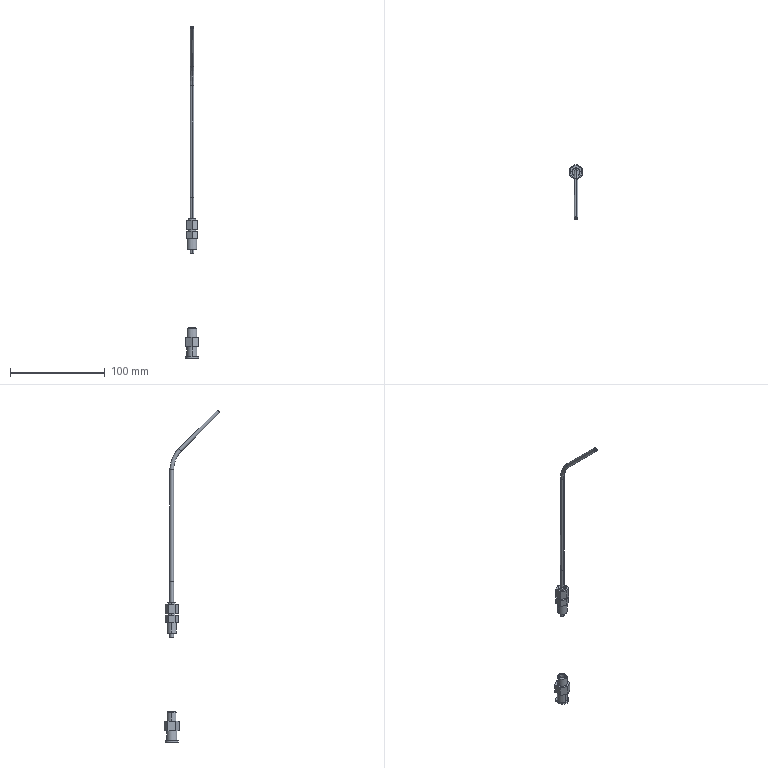Part | SolidWorks | features ICE 8, MoveCopyBody 2, Chamfer 1, MirrorSolid 1, WeldMemberFeat 1, WeldmentFeature 1 | 8 solids | 77 faces | box 14 x 58.995 x 350.912 mm | volume 7220 mm3 | plane 39 | cylinder 32 | torus 4 | cone 2 | commonest cylinder face diameters 4 x8 2 x6 10 x6 8 x4 6 x2 8.6 x2